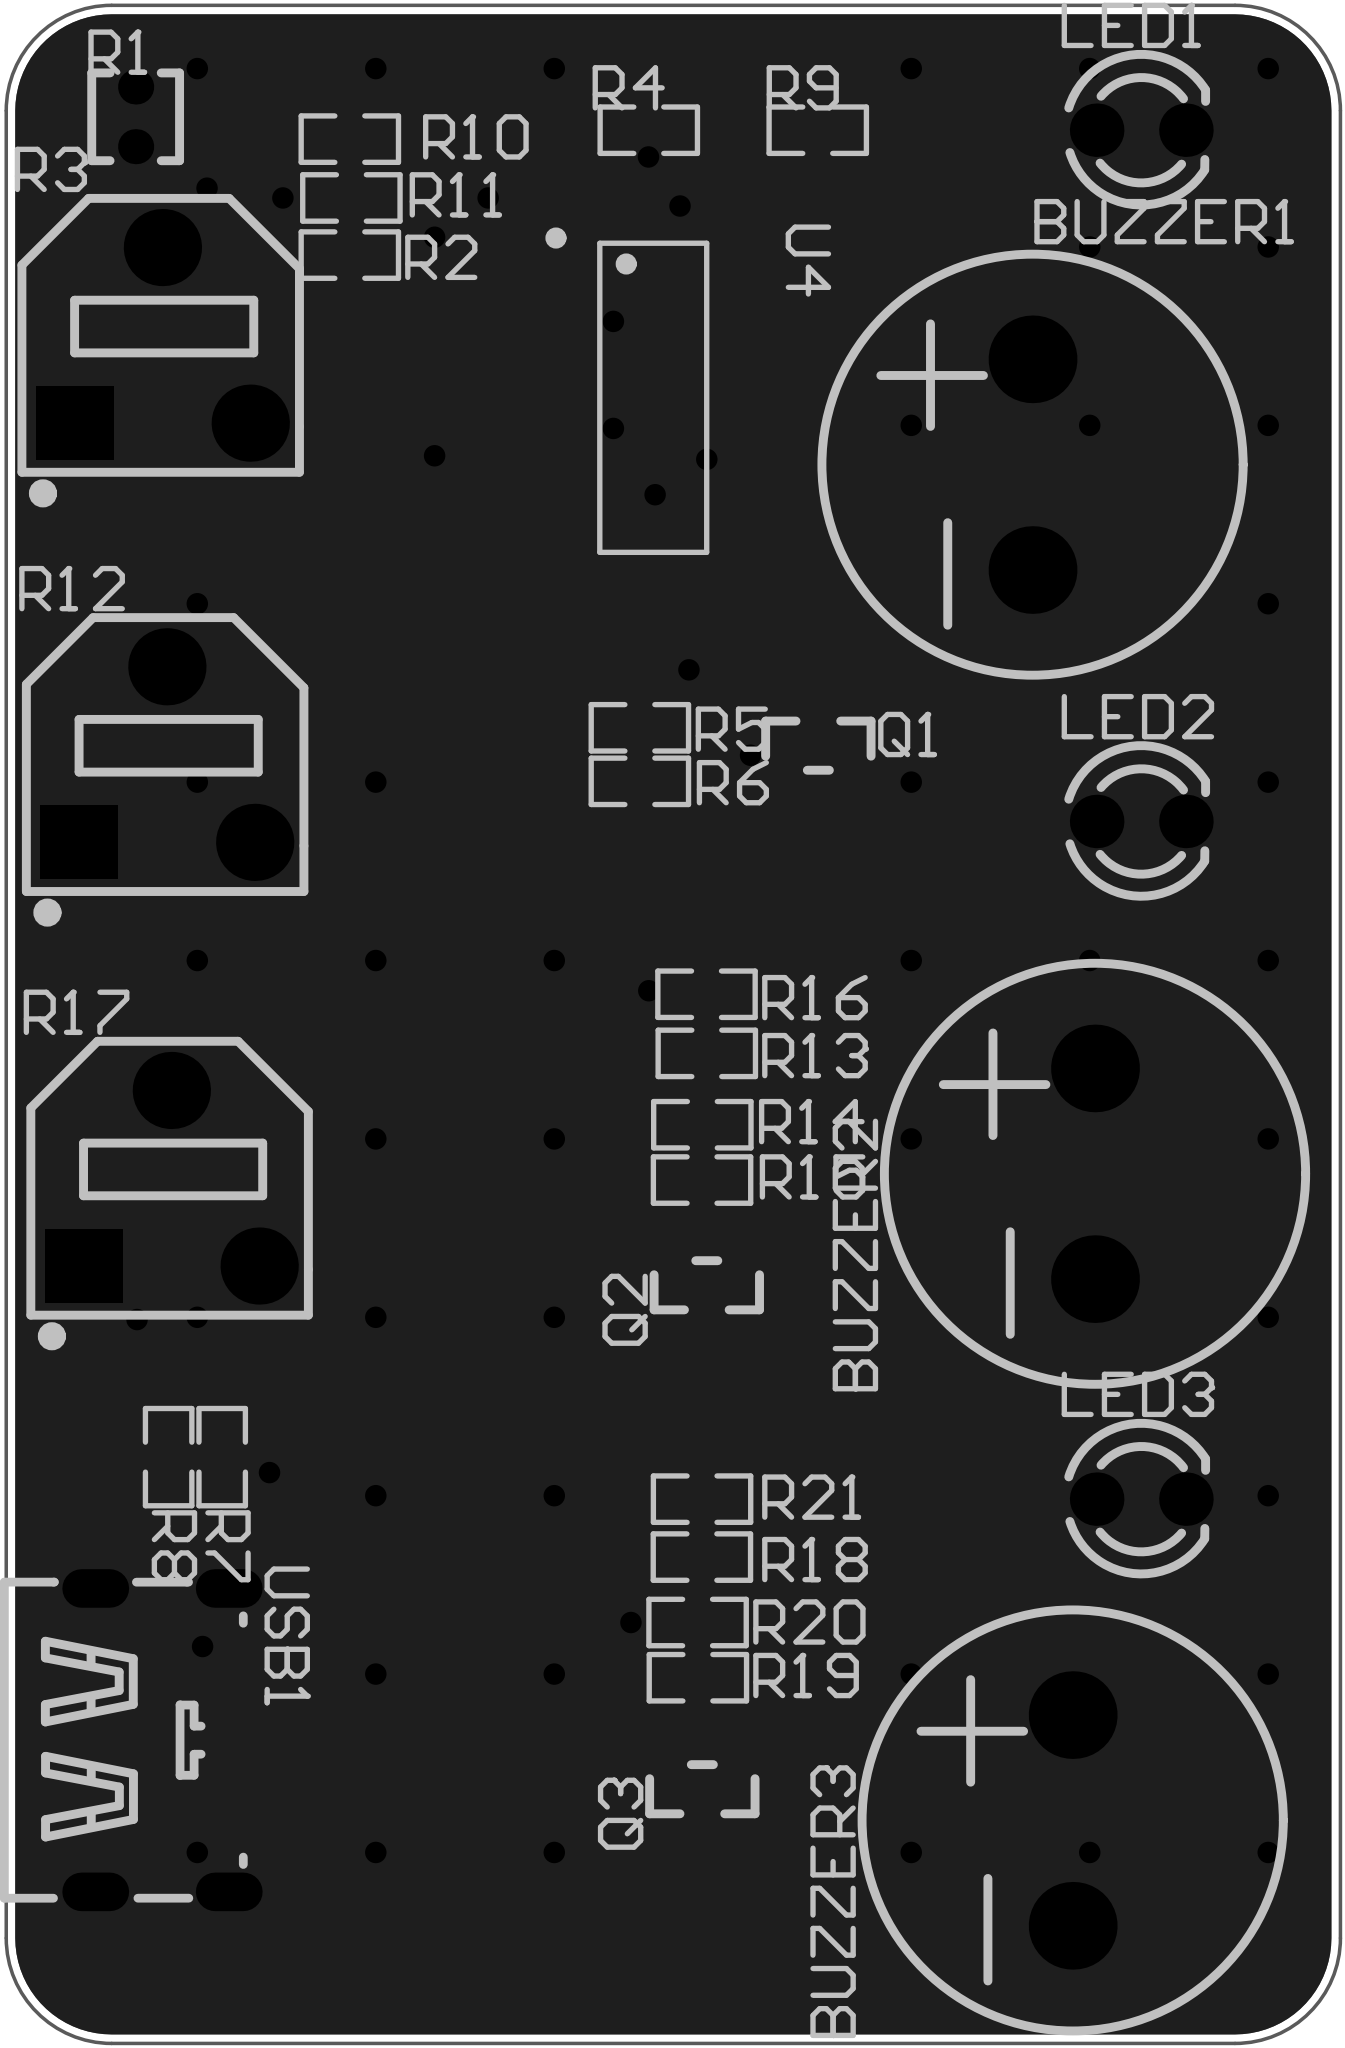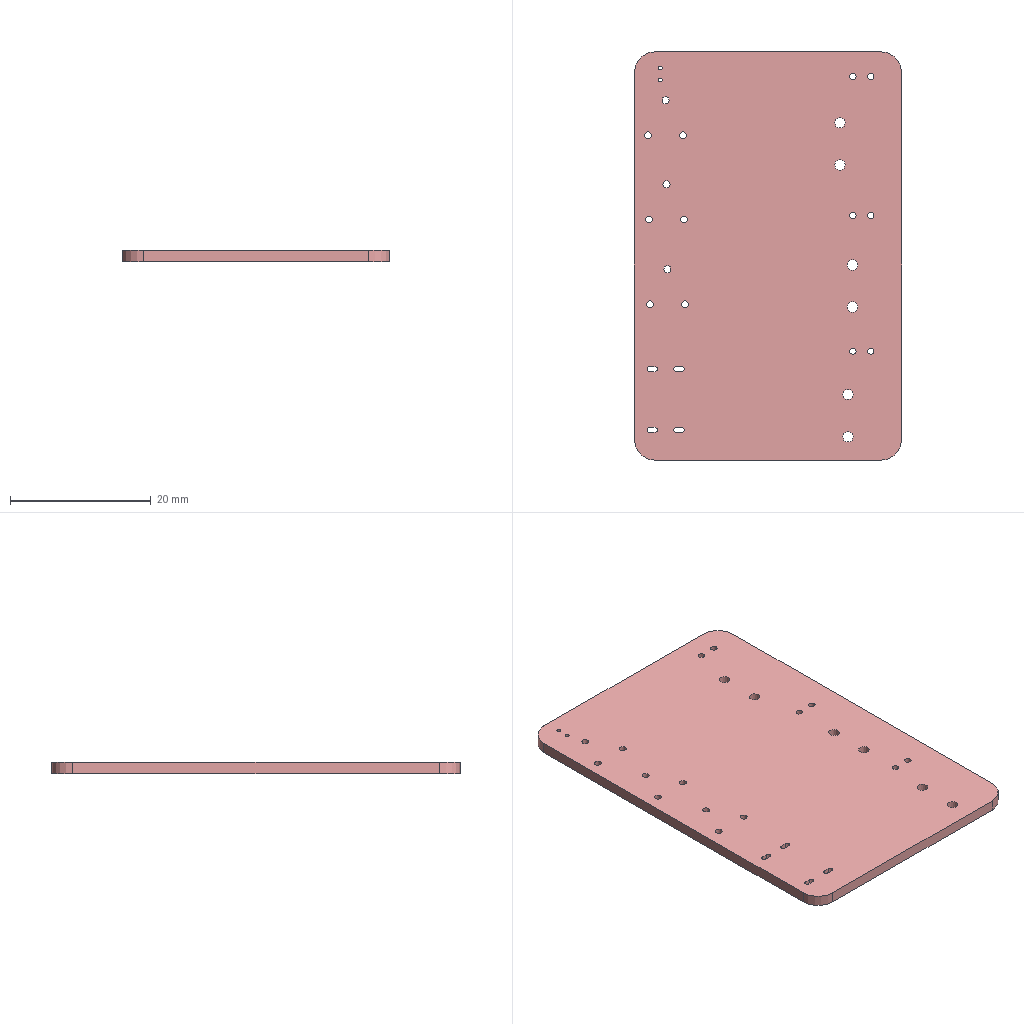Circuit board layout | Altium Designer | box 38 x 58 x 1.6 mm
Layer stack:
# Altium Designer layer stack of  (unit mm; dielectric type: 0 none, 1 core, 2 prepreg, 3 surface material)
index,name,kind,layer,copper_thickness_mm,dielectric_type,dielectric_thickness_mm,dielectric_material,dielectric_constant
0,Top Paste Mask Layer,other,,,,,,
1,Top Silkscreen Layer,other,,,,,,
2,Top Solder Mask Layer,dielectric,,,3,0.01,,3.3
3,Top Layer,copper,Top Layer,0.035,,,,
4,Dielectric1,dielectric,,,3,1.51,FR4,4.5
5,Bottom Layer,copper,Bottom Layer,0.035,,,,
6,Bottom Solder Mask Layer,dielectric,,,3,0.01,,3.3
7,Bottom Silkscreen Layer,other,,,,,,
8,Bottom Paste Mask Layer,other,,,,,,
# drill layer pairs: low layer,high layer
drill_pair,Top Layer,Bottom Layer
Part placement:
Designator,Comment,Layer,Footprint,Center-X(mm),Center-Y(mm),Rotation
BUZZER1,buzzer,TopLayer,BUZ-TH_BD12.0-P6.00-D0.9-RD,110.236,127.635,90
LED1,,TopLayer,LED_TH-3mm,113.331,137.16,0
Q1,,TopLayer,S8050_SOT-23,104.14,119.634,270
R1,MF52A503F3950 (A1),TopLayer,RES-TH_L2.5-W2.5-P1.70-D0.3,84.709,137.541,270
R2,1K,TopLayer,R0603,90.805,133.604,0
R3,10kΩ,TopLayer,RES-ADJ-SMD_RM065-V1,85.471,131.318,0
R4,10K,TopLayer,R0603,99.314,137.16,0
R5,1K,TopLayer,R0603,99.06,120.142,180
R6,10K,TopLayer,R0603,99.06,118.618,180
R7,5.1K,TopLayer,R0603,87.172,99.373,270
R8,5.1K,TopLayer,R0603,85.648,99.373,270
USB1,TYPE-C-6P-DIP2X2,TopLayer,TYPE-C-SMD_TYPE-C-6P,85.598,91.313,270
R9,100,TopLayer,R0603,104.123,137.16,180
BUZZER2,buzzer,TopLayer,BUZ-TH_BD12.0-P6.00-D0.9-RD,112.014,107.442,90
BUZZER3,buzzer,TopLayer,BUZ-TH_BD12.0-P6.00-D0.9-RD,111.379,89.027,90
LED2,,TopLayer,LED_TH-3mm,113.331,117.475,0
LED3,,TopLayer,LED_TH-3mm,113.331,98.177,0
Q2,,TopLayer,S8050_SOT-23,100.965,104.267,90
Q3,,TopLayer,S8050_SOT-23,100.838,89.916,90
R10,1K,TopLayer,R0603,90.805,136.906,0
R11,1K,TopLayer,R0603,90.85,135.231,180
R12,10kΩ,TopLayer,RES-ADJ-SMD_RM065-V1,85.598,119.38,0
R13,10K,TopLayer,R0603,100.965,110.871,0
R14,1K,TopLayer,R0603,100.838,108.839,180
R15,10K,TopLayer,R0603,100.83,107.264,180
R16,100,TopLayer,R0603,100.957,112.555,180
R17,10kΩ,TopLayer,RES-ADJ-SMD_RM065-V1,85.725,107.315,0
R18,10K,TopLayer,R0603,100.825,96.527,0
R19,1K,TopLayer,R0603,100.711,93.091,180
R20,10K,TopLayer,R0603,100.703,94.663,180
R21,100,TopLayer,R0603,100.83,98.177,180
U4,LM324DT,TopLayer,SOIC-14_L8.7-W3.9-P1.27-LS6.0-BL,99.441,129.54,270
Pad and via stacks:
# Altium Designer via and pad stacks of  (unit mm). Each distinct definition once, with the count of objects using it.
# via: kind,start_layer,end_layer,hole_mm,diameter_mm,mode(0 simple;1 top-mid-bottom;2 full stack),diameter_per_layer,count,example_net
# pad: kind,layer,hole_mm,hole_type(0 round;1 square;2 slot),plating,top_size,top_shape(1 round;2 rect;3 octagon;9 rounded rect),mid_size,bottom_size,mode,footprint,size_per_layer,count,example
pad,Multi-Layer,1.5,0,plated,2.5x2.5,1,2.5x2.5,2.5x2.5,0,BUZ-TH_BD12.0-P6.00-D0.9-RD,,6,BUZZER1.1
pad,Multi-Layer,0.9144,0,plated,1.524x1.524,1,1.524x1.524,1.524x1.524,0,LED_TH-3mm,,6,LED1.1
pad,Multi-Layer,0.55,0,plated,1x1,1,1x1,1x1,0,RES-TH_L2.5-W2.5-P1.70-D0.3,,2,R1.1
pad,Multi-Layer,1,0,plated,2.2x2.1,2,2.2x2.1,2.2x2.1,0,RES-ADJ-SMD_RM065-V1,,3,R3.1
pad,Multi-Layer,1,0,plated,2.2x2.2,1,2.2x2.2,2.2x2.2,0,RES-ADJ-SMD_RM065-V1,,6,R3.3
pad,Multi-Layer,0.7,2,plated,1.1x1.9,1,1.1x1.9,1.1x1.9,0,TYPE-C-SMD_TYPE-C-6P,,4,USB1.7
pad,Top Layer,0,0,plated,1x0.8,2,1x0.8,1x0.8,0,S8050_SOT-23,,9,Q1.2
pad,Top Layer,0,0,plated,0.8065x0.864,2,0.8065x0.864,0.8065x0.864,0,R0603,,34,R2.2
pad,Top Layer,0,0,plated,0.8x1.2,2,0.8x1.2,0.8x1.2,0,TYPE-C-SMD_TYPE-C-6P,,2,USB1.B12
pad,Top Layer,0,0,plated,0.7x1.2,2,0.7x1.2,0.7x1.2,0,TYPE-C-SMD_TYPE-C-6P,,4,USB1.B9
pad,Top Layer,0,0,plated,0.574x2.038,1,0.574x2.038,0.574x2.038,0,SOIC-14_L8.7-W3.9-P1.27-LS6.0-BL,,14,U4.1
via,Top Layer,Bottom Layer,0.3048,0.61,0,,60,$1N1542
via,Top Layer,Bottom Layer,0.3048,0.6096,0,,2,GND
Copper pours:
name,layer,net,type(0 solid;1 hatched;2 none)
Top Layer-GND,Top Layer,GND,0
Bottom Layer-GND,Bottom Layer,GND,0
Design rules, without the lines most boards share:
# Altium Designer design rules of  (exported by Altium Designer, unit mm)
# columns: name | kind | enabled | priority | scope1 | scope2 | descriptor | typed fields (field=value)
copperThickness1oz_2 | 2 | enabled | 2 | All | All | Width Constraint (Min=5mil) (Max=100mil) (Preferred=30mil) (All) |
viaSize | 11 | enabled | 1 | All | All | Routing Via (MinHoleWidth=11.811mil) (MaxHoleWidth=248.032mil) (PreferredHoleWidth=12.008mil) (MinWidth=19.685mil) (MaxWidth=393.701mil) (PreferedWidth=24.016mil) (All) | via_min_hole=0.3 via_max_hole=6.3 via_preferred_diameter=0.61 via_preferred_hole=0.305
solderMaskExpansion | 13 | enabled | 2 | All | All | Solder Mask Expansion (Expansion =2.008mil) (All) | expansion=0.051